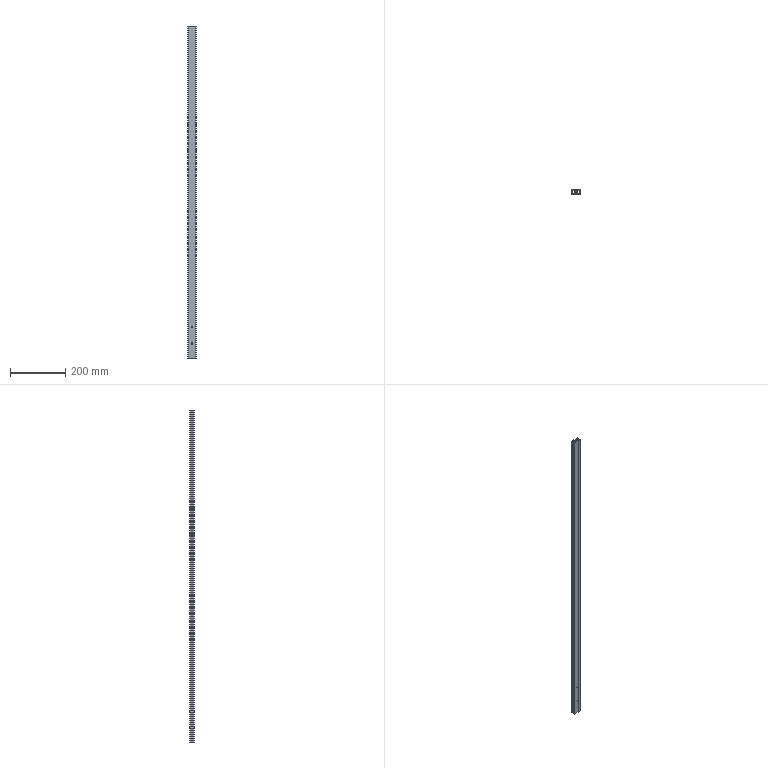Part | SolidWorks | features BaseBody 1, HoleWzd 1, MoveFace 1 | 1 solid | 87 faces | box 30 x 15 x 1200 mm | volume 289001 mm3 | plane 46 | cylinder 41 | commonest cylinder face diameters 5 x31 1 x6 2 x4